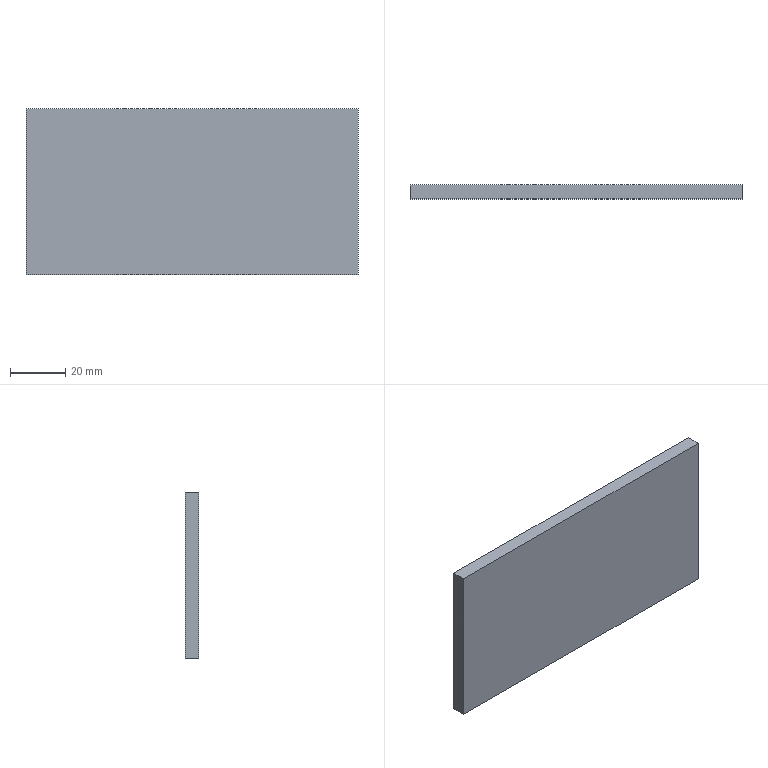Part | SolidWorks | features Extrusion 1 | 1 solid | 6 faces | box 120 x 5 x 60 mm | volume 36000 mm3 | plane 6
STEP:
#1=CARTESIAN_POINT('',(60.,0.,30.));
#2=VERTEX_POINT('',#1);
#3=CARTESIAN_POINT('',(60.,0.,-30.));
#4=VERTEX_POINT('',#3);
#5=CARTESIAN_POINT('',(60.,0.,-30.));
#6=DIRECTION('',(0.,0.,-1.));
#7=VECTOR('',#6,1000.);
#8=LINE('',#5,#7);
#9=EDGE_CURVE('',#2,#4,#8,.T.);
#10=ORIENTED_EDGE('',*,*,#9,.T.);
#11=CARTESIAN_POINT('',(60.,5.,-30.));
#12=VERTEX_POINT('',#11);
#13=CARTESIAN_POINT('',(60.,5.,-30.));
#14=DIRECTION('',(0.,-1.,0.));
#15=VECTOR('',#14,1000.);
#16=LINE('',#13,#15);
#17=EDGE_CURVE('',#12,#4,#16,.T.);
#18=ORIENTED_EDGE('',*,*,#17,.F.);
#19=CARTESIAN_POINT('',(60.,5.,30.));
#20=VERTEX_POINT('',#19);
#21=CARTESIAN_POINT('',(60.,5.,-30.));
#22=DIRECTION('',(0.,0.,-1.));
#23=VECTOR('',#22,1000.);
#24=LINE('',#21,#23);
#25=EDGE_CURVE('',#20,#12,#24,.T.);
#26=ORIENTED_EDGE('',*,*,#25,.F.);
#27=CARTESIAN_POINT('',(60.,5.,30.));
#28=DIRECTION('',(0.,-1.,0.));
#29=VECTOR('',#28,1000.);
#30=LINE('',#27,#29);
#31=EDGE_CURVE('',#20,#2,#30,.T.);
#32=ORIENTED_EDGE('',*,*,#31,.T.);
#33=EDGE_LOOP('',(#10,#18,#26,#32));
#34=FACE_OUTER_BOUND('',#33,.T.);
#35=CARTESIAN_POINT('',(60.,5.,-30.));
#36=DIRECTION('',(-1.,0.,0.));
#37=DIRECTION('',(0.,0.,1.));
#38=AXIS2_PLACEMENT_3D('',#35,#36,#37);
#39=PLANE('',#38);
#40=ADVANCED_FACE('',(#34),#39,.F.);
#41=CARTESIAN_POINT('',(-60.,0.,-30.));
#42=VERTEX_POINT('',#41);
#43=CARTESIAN_POINT('',(-60.,0.,-30.));
#44=DIRECTION('',(-1.,0.,0.));
#45=VECTOR('',#44,1000.);
#46=LINE('',#43,#45);
#47=EDGE_CURVE('',#4,#42,#46,.T.);
#48=ORIENTED_EDGE('',*,*,#47,.T.);
#49=CARTESIAN_POINT('',(-60.,5.,-30.));
#50=VERTEX_POINT('',#49);
#51=CARTESIAN_POINT('',(-60.,5.,-30.));
#52=DIRECTION('',(0.,-1.,0.));
#53=VECTOR('',#52,1000.);
#54=LINE('',#51,#53);
#55=EDGE_CURVE('',#50,#42,#54,.T.);
#56=ORIENTED_EDGE('',*,*,#55,.F.);
#57=CARTESIAN_POINT('',(-60.,5.,-30.));
#58=DIRECTION('',(-1.,0.,0.));
#59=VECTOR('',#58,1000.);
#60=LINE('',#57,#59);
#61=EDGE_CURVE('',#12,#50,#60,.T.);
#62=ORIENTED_EDGE('',*,*,#61,.F.);
#63=ORIENTED_EDGE('',*,*,#17,.T.);
#64=EDGE_LOOP('',(#48,#56,#62,#63));
#65=FACE_OUTER_BOUND('',#64,.T.);
#66=CARTESIAN_POINT('',(-60.,5.,-30.));
#67=DIRECTION('',(0.,0.,1.));
#68=DIRECTION('',(1.,0.,0.));
#69=AXIS2_PLACEMENT_3D('',#66,#67,#68);
#70=PLANE('',#69);
#71=ADVANCED_FACE('',(#65),#70,.F.);
#72=CARTESIAN_POINT('',(-60.,0.,30.));
#73=VERTEX_POINT('',#72);
#74=CARTESIAN_POINT('',(-60.,0.,-30.));
#75=DIRECTION('',(0.,0.,1.));
#76=VECTOR('',#75,1000.);
#77=LINE('',#74,#76);
#78=EDGE_CURVE('',#42,#73,#77,.T.);
#79=ORIENTED_EDGE('',*,*,#78,.T.);
#80=CARTESIAN_POINT('',(-60.,5.,30.));
#81=VERTEX_POINT('',#80);
#82=CARTESIAN_POINT('',(-60.,5.,30.));
#83=DIRECTION('',(0.,-1.,0.));
#84=VECTOR('',#83,1000.);
#85=LINE('',#82,#84);
#86=EDGE_CURVE('',#81,#73,#85,.T.);
#87=ORIENTED_EDGE('',*,*,#86,.F.);
#88=CARTESIAN_POINT('',(-60.,5.,-30.));
#89=DIRECTION('',(0.,0.,1.));
#90=VECTOR('',#89,1000.);
#91=LINE('',#88,#90);
#92=EDGE_CURVE('',#50,#81,#91,.T.);
#93=ORIENTED_EDGE('',*,*,#92,.F.);
#94=ORIENTED_EDGE('',*,*,#55,.T.);
#95=EDGE_LOOP('',(#79,#87,#93,#94));
#96=FACE_OUTER_BOUND('',#95,.T.);
#97=CARTESIAN_POINT('',(-60.,5.,-30.));
#98=DIRECTION('',(1.,0.,0.));
#99=DIRECTION('',(0.,0.,-1.));
#100=AXIS2_PLACEMENT_3D('',#97,#98,#99);
#101=PLANE('',#100);
#102=ADVANCED_FACE('',(#96),#101,.F.);
#103=CARTESIAN_POINT('',(-60.,0.,30.));
#104=DIRECTION('',(1.,0.,0.));
#105=VECTOR('',#104,1000.);
#106=LINE('',#103,#105);
#107=EDGE_CURVE('',#73,#2,#106,.T.);
#108=ORIENTED_EDGE('',*,*,#107,.T.);
#109=ORIENTED_EDGE('',*,*,#31,.F.);
#110=CARTESIAN_POINT('',(-60.,5.,30.));
#111=DIRECTION('',(1.,0.,0.));
#112=VECTOR('',#111,1000.);
#113=LINE('',#110,#112);
#114=EDGE_CURVE('',#81,#20,#113,.T.);
#115=ORIENTED_EDGE('',*,*,#114,.F.);
#116=ORIENTED_EDGE('',*,*,#86,.T.);
#117=EDGE_LOOP('',(#108,#109,#115,#116));
#118=FACE_OUTER_BOUND('',#117,.T.);
#119=CARTESIAN_POINT('',(-60.,5.,30.));
#120=DIRECTION('',(0.,0.,-1.));
#121=DIRECTION('',(-1.,0.,0.));
#122=AXIS2_PLACEMENT_3D('',#119,#120,#121);
#123=PLANE('',#122);
#124=ADVANCED_FACE('',(#118),#123,.F.);
#125=ORIENTED_EDGE('',*,*,#25,.T.);
#126=ORIENTED_EDGE('',*,*,#61,.T.);
#127=ORIENTED_EDGE('',*,*,#92,.T.);
#128=ORIENTED_EDGE('',*,*,#114,.T.);
#129=EDGE_LOOP('',(#125,#126,#127,#128));
#130=FACE_OUTER_BOUND('',#129,.T.);
#131=CARTESIAN_POINT('',(0.,5.,0.));
#132=DIRECTION('',(0.,1.,0.));
#133=DIRECTION('',(0.,0.,1.));
#134=AXIS2_PLACEMENT_3D('',#131,#132,#133);
#135=PLANE('',#134);
#136=ADVANCED_FACE('',(#130),#135,.T.);
#137=ORIENTED_EDGE('',*,*,#9,.F.);
#138=ORIENTED_EDGE('',*,*,#107,.F.);
#139=ORIENTED_EDGE('',*,*,#78,.F.);
#140=ORIENTED_EDGE('',*,*,#47,.F.);
#141=EDGE_LOOP('',(#137,#138,#139,#140));
#142=FACE_OUTER_BOUND('',#141,.T.);
#143=CARTESIAN_POINT('',(0.,0.,0.));
#144=DIRECTION('',(0.,1.,0.));
#145=DIRECTION('',(0.,0.,1.));
#146=AXIS2_PLACEMENT_3D('',#143,#144,#145);
#147=PLANE('',#146);
#148=ADVANCED_FACE('',(#142),#147,.F.);
#149=CLOSED_SHELL('',(#40,#71,#102,#124,#136,#148));
#150=MANIFOLD_SOLID_BREP('',#149);
#151=CARTESIAN_POINT('',(0.,0.,0.));
#152=DIRECTION('',(0.,0.,1.));
#153=DIRECTION('',(1.,0.,0.));
#154=AXIS2_PLACEMENT_3D('',#151,#152,#153);
#155=(LENGTH_UNIT()NAMED_UNIT(*)SI_UNIT(.MILLI.,.METRE.));
#156=UNCERTAINTY_MEASURE_WITH_UNIT(LENGTH_MEASURE(0.00001),#155,'','');
#157=(NAMED_UNIT(*)PLANE_ANGLE_UNIT()SI_UNIT($,.RADIAN.));
#158=(NAMED_UNIT(*)SI_UNIT($,.STERADIAN.)SOLID_ANGLE_UNIT());
#159=(GEOMETRIC_REPRESENTATION_CONTEXT(3)GLOBAL_UNCERTAINTY_ASSIGNED_CONTEXT((#156))GLOBAL_UNIT_ASSIGNED_CONTEXT((#155,#157,#158))REPRESENTATION_CONTEXT('',''));
#160=ADVANCED_BREP_SHAPE_REPRESENTATION('',(#150,#154),#159);